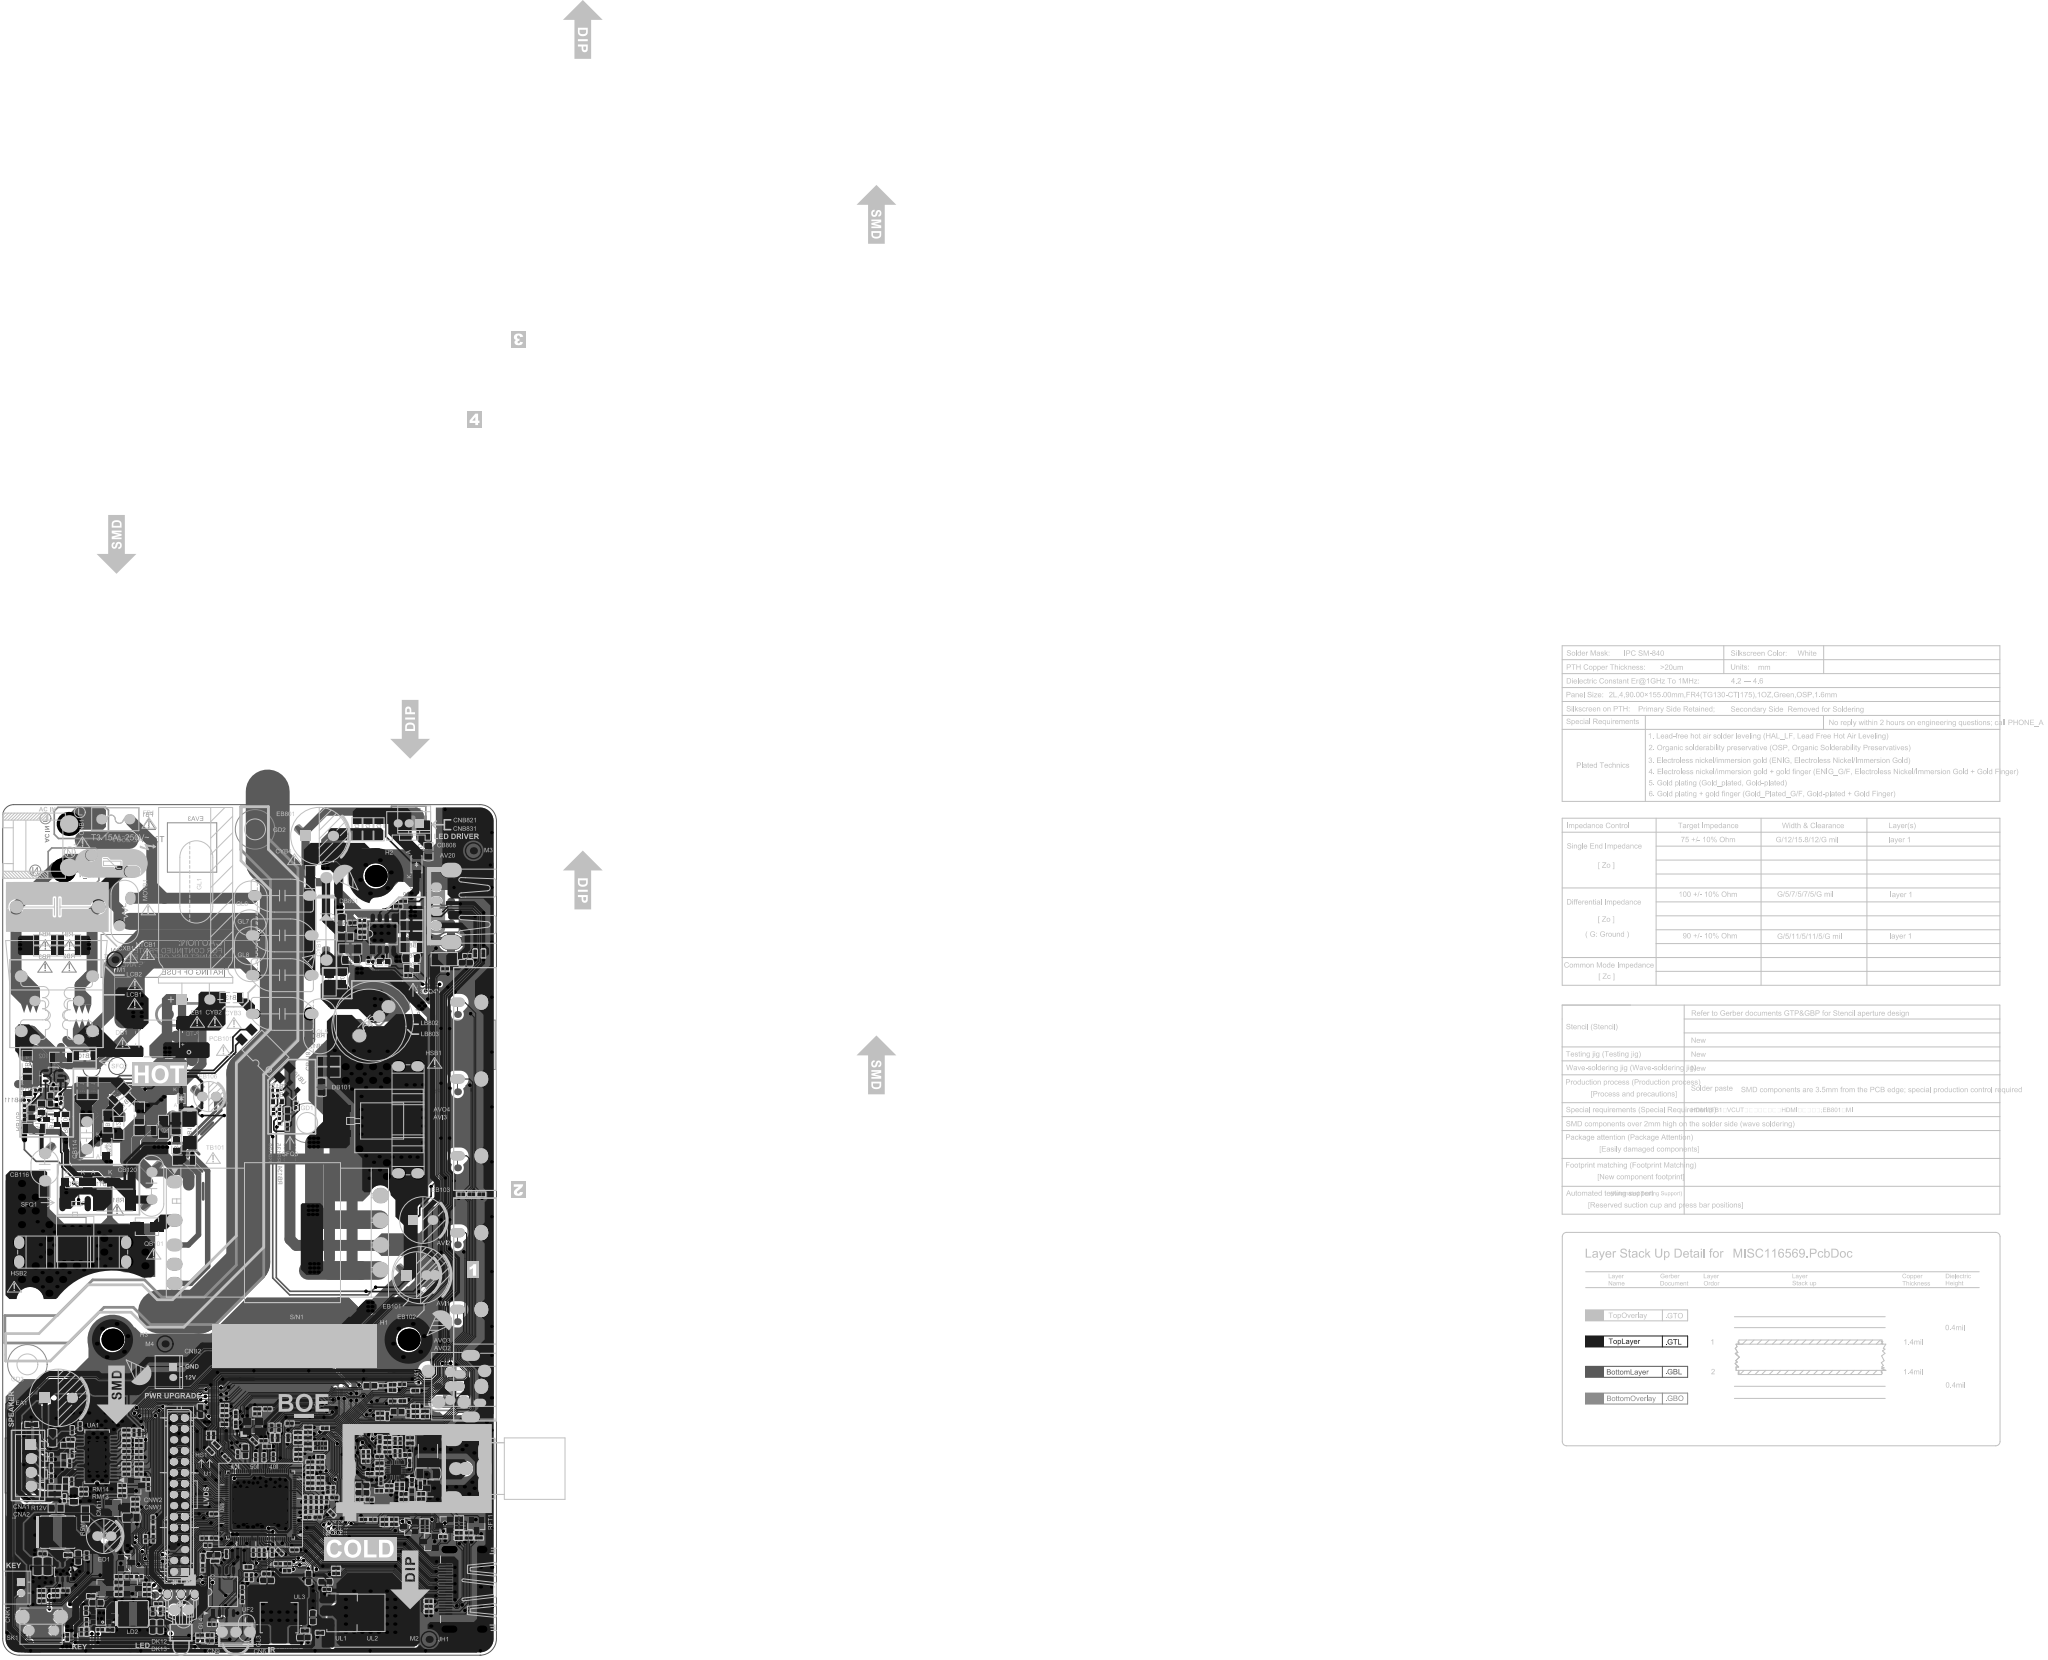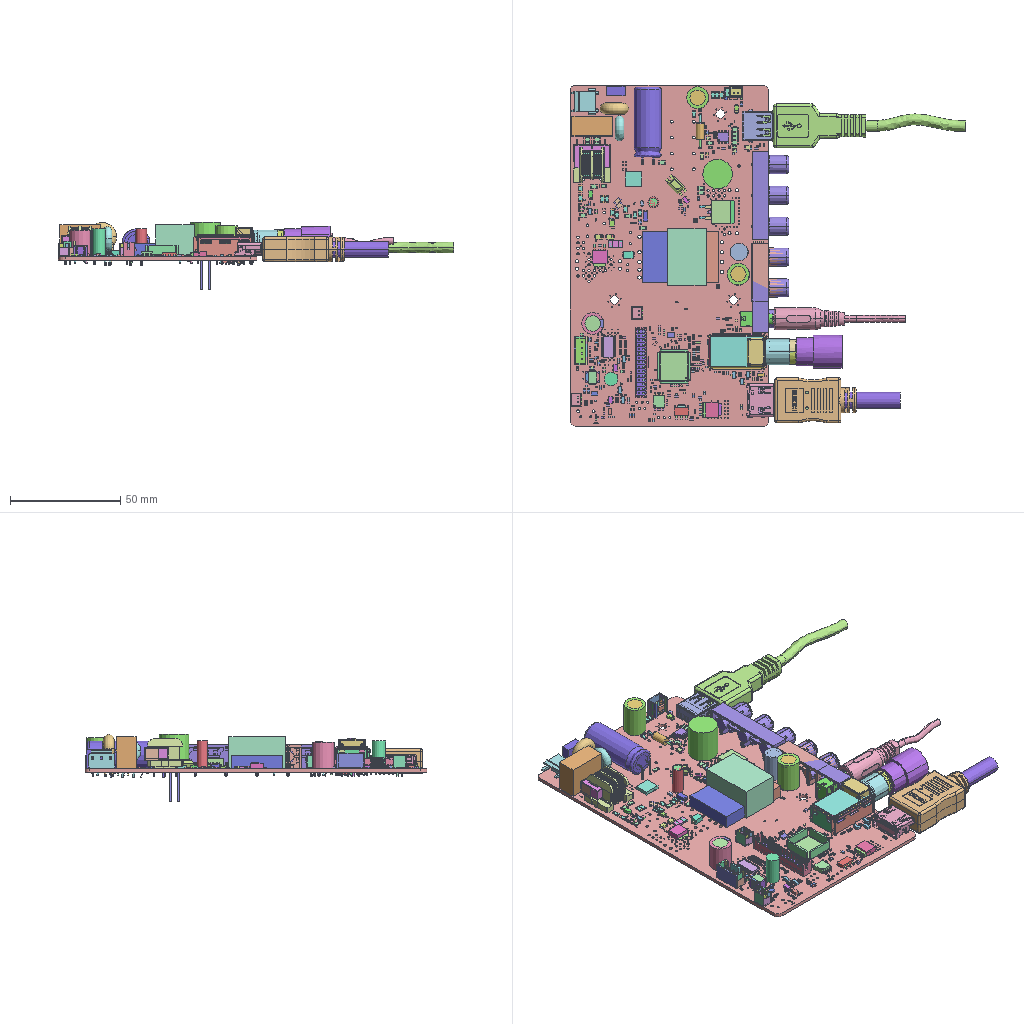Circuit board layout | Altium Designer | box 179.2 x 155 x 30.5 mm
Layer stack:
# Altium Designer layer stack of  (unit mm; dielectric type: 0 none, 1 core, 2 prepreg, 3 surface material)
index,name,kind,layer,copper_thickness_mm,dielectric_type,dielectric_thickness_mm,dielectric_material,dielectric_constant
0,TopPaste,other,,,,,,
1,TopOverlay,other,,,,,,
2,TopSolder,dielectric,,,3,0.0102,Solder Resist,3.5
3,TopLayer,copper,TopLayer,0.0356,,,,
4,Dielectric1,dielectric,,,1,1.5,FR-4,4.8
5,BottomLayer,copper,BottomLayer,0.0356,,,,
6,BottomSolder,dielectric,,,3,0.0102,Solder Resist,3.5
7,BottomOverlay,other,,,,,,
8,BottomPaste,other,,,,,,
# drill layer pairs: low layer,high layer
drill_pair,TopLayer,BottomLayer
Part placement, first 334 of 528 lines:
Designator,Comment,Layer,Footprint,Center-X(mm),Center-Y(mm),Rotation
DBS8,DOLBY Double-D,BottomLayer,Double-D-SILK,-1655.786,-747.429,180
M4,MARK,TopLayer,MARK,29.604,56.731,0
M1,MARK,TopLayer,MARK,20.475,126.729,0
GL4,Silicone,0.5g,general purpose,60,White,SLD-8854W,XY,TopLayer,Silica_gel-5*3,-1655.786,-747.429,0
GL3,Silicone,0.5g,general purpose,60,White,SLD-8854W,XY,TopLayer,Silica_gel-5*3,-1655.786,-747.429,0
SFQ4,NC/Conformal coating,25kg/Can,Peters,TopLayer,SFQ,-1655.786,-747.429,90
SFQ3,NC/Conformal coating,25kg/Can,Peters,TopLayer,SFQ,-1655.786,-747.429,90
SFQ2,NC/Conformal coating,25kg/Can,Peters,TopLayer,SFQ,-1655.786,-747.429,180
SFQ1,NC/Conformal coating,25kg/Can,Peters,TopLayer,SFQ,-1655.786,-747.429,0
GL6,NC/Silicone,0.5g,general purpose,60,White,SLD-8854W,XY,TopLayer,Silica_gel-10,-1655.786,-747.429,0
GL5,NC/Silicone,0.5g,general purpose,60,White,SLD-8854W,XY,TopLayer,Silica_gel-10,-1655.786,-747.429,180
GL8,NC/Silicone,0.5g,general purpose,60,White,SLD-8854W,XY,TopLayer,Silica_gel-10,-1655.786,-747.429,0
GL7,NC/Silicone,0.5g,general purpose,60,White,SLD-8854W,XY,TopLayer,Silica_gel-10,-1655.786,-747.429,0
CB808,220PF-0805-NPO-±10%-200V,TopLayer,C0805,77.597,146.468,90
CYB4,Y capacitor,CAP Y1,CD,100pF,400VAC,±10%,K,10mm,Y5P,DIP,TP,TDK,TopLayer,CAP13*5-V-10-1,50.964,138.428,360
RB5,NC/Thick-film resistor,RES,1/4W,0ohm,±5%,1206,SMD,TopLayer,R1206SC,56.071,141.798,90
FBA2,NC/0ohm-0603-PCB,TopLayer,R0603SC,5.271,42.024,180
FBA1,NC/0ohm-0603-PCB,TopLayer,R0603SC,9.481,29.401,180
RB109,10Kohm-0402-±1%-1/16W,TopLayer,R0402,13.399,82.283,180
QM12,MOSFET,PMOS,-4.3A,-30V,0.048ohm@ID=-3A@VGS=-4.5V,SOT-23-3L,NCE3407AY,NCEPOWER,TopLayer,SOT-23-1,20.531,26.835,90
TB101,变压器,Transformer,EQ2414,300uH,0.2×1P,26Ts,H14.5MAX,SYEQ2414Z-T012064B(BLACK),DIP,SQ,TopLayer,T/EQ2414*10,50.073,77.006,360
CA26,2200pF-0402-X7R-±10%-50V,TopLayer,C0402,8.877,34.096,90
RK3,1Kohm-0402-±1%-1/16W,TopLayer,R0402,44.42,14.226,270
DU4,NC/Thick-film resistor,TVS diode,DIO ESD,0.1pF,25V,0402,SMD,GESD1005H150CR10GPT,Sunlord,TopLayer,DIODE-S0402,37.841,37.213,315
??U1?,NC/Glue,0.1g,silicone,ZJ,TopLayer,Heat-Shrinkable_Tube,35.865,5.359,90
YPBPR_R/AV_R,DM0,BottomLayer,TP,82.875,74.793,90
YPBPR_L/AV_L,DM0,BottomLayer,TP,82.85,60.785,90
Y_Y_AV_OUT,DM0,BottomLayer,TP,82.901,88.814,90
Y_Pr_ROUT,DM0,BottomLayer,TP,82.901,116.766,90
Y_Pb_LOUT,DM0,BottomLayer,TP,82.901,102.669,90
UL2,NC/LC1117COTR33,TopLayer,TO-252,62.68,7.728,270
UL1,LDO regulator,IC LDO,1A,3.3V,15V,SOT223,SMD,SCJT1117B-3.3V,CJKJ,TopLayer,SOT-223,61.83,7.728,270
UD2,DC-DC converter,IC DCDC,Syn,1.2A,6.0V,1.5MHz,SOT23-5,SMD,TMI3408,TOLL,TopLayer,SOT-23-5,17.899,6.975,90
UD1,DC-DC converter,IC DC-DC,Syn,3A,18V,600KHz,SOT23-6,SMD,TMI3253T,TOLL,TopLayer,TSOT23-6,10.917,15.175,270
UB801,PWM controller,IC PWM Controller,120KHz,SOP-8,SMD,OB33510CPA,ON-Bright,TopLayer,SO-8A,69.362,131.458,90
UB101,PWM controller,IC PWM Controller,100KHZ,SOT23-6,SMD,LD5537B3GL,Leadtrend,TopLayer,SOT-26,9.207,105.6,270
UART_RX,,BottomLayer,TP,72.873,23.254,180
SK1,Tact switch,Tact Switch,160±50gf,7.0×10.3×7.0mm,DIP,106520070,VAST,TopLayer,KEY-HD-6,6.996,5.75,0
RU4,Thick-film resistor,RES,1/16W,0ohm,±1%,0402,SMD,TopLayer,R0402,80.64,125.07,180
RT15,Thick-film resistor,RES,1/16W,100ohm,±1%,0402,SMD,TopLayer,R0402,72.436,39.048,90
RT14,Thick-film resistor,RES,1/16W,100ohm,±1%,0402,SMD,TopLayer,R0402,71.521,39.048,90
RT10,Thick-film resistor,RES,1/16W,100ohm,±1%,0402,SMD,TopLayer,R0402,65.724,36.676,90
RPV7,Resistor array,RES ARRAY,1/16W,4×4.7Kohm,±5%,0402,SMD,TopLayer,RA0402,76.901,23.608,360
RPV5,Resistor array,RES ARRAY,1/16W,4×10Kohm,±5%,0402,SMD,TopLayer,RA0402,57.937,38.199,90
RO18,NC/Thick-film resistor,RES,1/16W,75ohm,±1%,0402,SMD,TopLayer,R0402,56.071,34.194,180
RO17,NC/0ohm-0402-±5%-1/16W,TopLayer,R0402,57.868,35.204,360
RM4,Thick-film resistor,RES,1/16W,100Kohm,±1%,0402,SMD,TopLayer,R0402,23.055,14.313,180
RM3,4K7ohm-0402-±1%-1/16W,TopLayer,R0402,24.842,14.313,180
RM2,4K7ohm-0402-±1%-1/16W,TopLayer,R0402,21.135,14.313,180
RK19,1Kohm-0402-±1%-1/16W,TopLayer,R0402,36.482,15.941,90
RK18,22ohm-0402-±1%-1/16W,TopLayer,R0402,35.981,2.657,180
RI18,75ohm-0402-±1%-1/16W,TopLayer,R0402,57.921,32.334,180
RH89,100ohm-0402-±1%-1/16W,TopLayer,R0402,51.906,16.652,180
RH88,100ohm-0402-±1%-1/16W,TopLayer,R0402,71.305,24.778,360
RH59,1Kohm-0402-±1%-1/16W,TopLayer,R0402,80.234,21.605,180
RFT4,NC/RF shield can,RF SHLED,Single,H,F,T14.5,CH6.3,whole,25.0×14.5×10.0mm,DIP,T-14.5×25×10-F14.5-LHD,TopLayer,T-14.5¡Á25¡Á10-F14.5,75.5,34,90
RFT3,NC/T-25×14.5×9-IEC14.5-LHD (3 pins),TopLayer,T-25¡Á14.5¡Á9-IEC14.5-LHD-1,75.5,34,90
RFT2,NC/RF shield can,RF SHLED,Single,H,IEC,T14.5,CH6.3,whole,14.5×25×9,DIP,122010461,VAST,TopLayer,T-14.5¡Á25¡Á9.0-IEC14.5,75.5,34,90
RFT1,RF jack,RF JACK,H,IEC,T14.5,CH6.3,12.4×13.2×7.7mm,DIP,LHD-020 assembly,LHD,TopLayer,ANT-IEC14.5-H-4,84.825,34,90
RF25,Thick-film resistor,RES,1/16W,1.3Kohm,±1%,0402,SMD,TopLayer,R0402,46.376,43.97,180
RD9,Thick-film resistor,RES,1/16W,12Kohm,±1%,0402,SMD,TopLayer,R0402,14.308,4.27,90
RD8,Thick-film resistor,RES,1/16W,13Kohm,±1%,0402,SMD,TopLayer,R0402,15.261,6.083,90
RD7,Thick-film resistor,RES,1/16W,100Kohm,±1%,0402,SMD,TopLayer,R0402,17.782,4.638,180
RD6,NC/?,TopLayer,R0402,9.629,11.773,360
RD5,Thick-film resistor,RES,1/16W,10.5Kohm,±1%,0402,SMD,TopLayer,R0402,7.076,11.773,360
RD3,Thick-film resistor,RES,1/16W,60.4Kohm,±1%,0402,SMD,TopLayer,R0402,7.076,10.858,180
RD1,100Kohm-0402-±1%-1/16W,TopLayer,R0402,9.629,10.858,360
RB839,2R2ohm-1206-±1%-1/4W,TopLayer,R1206,68.591,150.512,270
RB838,2R2ohm-1206-±1%-1/4W,TopLayer,R1206,66.589,150.512,90
RB837,1R6ohm-1206-±1%-1/4W,TopLayer,R1206,64.586,150.512,90
RB820,0R1ohm-1206-±1%-1/4W,TopLayer,R1206,74.493,130.963,180
RB819,0R1ohm-1206-±1%-1/4W,TopLayer,R1206,74.493,132.946,180
RB818,0R2ohm-1206-±1%-1/4W,TopLayer,R1206,74.493,134.928,180
RB816,Thick-film resistor,RES,1/8W,10ohm,±1%,0805,SMD,TopLayer,R0805,74.557,125.146,180
RB814,Thick-film resistor,RES,1/8W,390Kohm,±1%,0805-Auto,SMD,TopLayer,R0805,62.505,130.899,180
RB812,Thick-film resistor,RES,1/4W,10ohm,±1%,1206,SMD,TopLayer,R1206,63.354,128.702,180
RB810,Thick-film resistor,RES,1/4W,10ohm,±1%,1206,SMD,TopLayer,R1206,74.493,128.981,360
RB805,Thick-film resistor,RES,1/16W,100ohm,±1%,0402,SMD,TopLayer,R0402,72.987,137.427,360
RB804,NC/10Kohm-0402-±5%-1/16W,TopLayer,R0402,65.54,133.922,180
RB803,10Kohm-0402-±1%-1/16W,TopLayer,R0402,65.54,130.835,360
RB801,Thick-film resistor,RES,1/16W,100ohm,±1%,0402,SMD,TopLayer,R0402,73.915,123.888,180
RB148,Thick-film resistor,RES,2W,0.36ohm,±5%,2512,SMD,TopLayer,R2512-1,20.434,82.944,180
RB135,18Kohm-0402-±1%-1/16W,TopLayer,R0402,50.516,99.092,270
RB134,4K7ohm-0402-±1%-1/16W,TopLayer,R0402,50.503,97.365,90
RB130,Thick-film resistor,RES,1/4W,20ohm,±1%,1206,SMD,TopLayer,R1206,41.689,119.842,360
RB128,Thick-film resistor,RES,1/4W,100Kohm,±1%,1206-Auto,SMD,TopLayer,R1206,22.123,100.457,45
RB127,Thick-film resistor,RES,1/4W,100Kohm,±1%,1206-Auto,SMD,TopLayer,R1206,21.161,96.094,90
RB126,Thick-film resistor,RES,1/4W,100Kohm,±1%,1206-Auto,SMD,TopLayer,R1206,21.285,102.413,45
RB125,Thick-film resistor,RES,1/4W,100Kohm,±1%,1206-Auto,SMD,TopLayer,R1206,19.168,97.262,90
RB124,47ohm-1206-±5%-1/4W,TopLayer,R1206,59.413,108.246,360
RB123,47ohm-1206-±5%-1/4W,TopLayer,R1206,59.413,106.265,360
RB118,Thick-film resistor,RES,1/4W,10ohm,±1%,1206,SMD,TopLayer,R1206,14.488,103.347,90
RB117,Thick-film resistor,RES,1/4W,10ohm,±1%,1206,SMD,TopLayer,R1206,16.472,103.347,90
RB116,NC/10ohm-1206-±5%-1/4W,TopLayer,R1206,31.598,96.926,270
RB114,4R7ohm-1206-±1%-1/4W,TopLayer,R1206,33.059,90.208,360
RB107,20ohm-0805-±5%-1/8W,TopLayer,R0805,7.087,99.682,270
RB106,68ohm-0805-±5%-1/8W,TopLayer,R0805,11.455,97.638,270
RB105,510ohm-0402-±1%-1/16W,TopLayer,R0402,3.975,97.987,270
RB103,6K8ohm-0402-±1%-1/16W,TopLayer,R0402,3.975,99.695,270
RB102,Thick-film resistor,RES,1/4W,330Kohm,±1%,1206,SMD,TopLayer,R1206,10.631,108.95,180
RB101,Thick-film resistor,RES,1/4W,330Kohm,±1%,1206,SMD,TopLayer,R1206,14.96,109.24,180
RB4,1M2ohm-1206-±5%-1/4W,TopLayer,R1206,7.73,130.345,180
RB3,1M2ohm-1206-±5%-1/4W,TopLayer,R1206,7.73,128.351,180
RB2,1M2ohm-1206-±5%-1/4W,TopLayer,R1206,12.103,128.347,180
RB1,1M2ohm-1206-±5%-1/4W,TopLayer,R1206,12.103,130.341,180
RA34,NC/Thick-film resistor,RES,1/16W,180ohm,±1%,0402,SMD,TopLayer,R0402,73.901,44.025,90
RA33,NC/Thick-film resistor,RES,1/16W,180ohm,±1%,0402,SMD,TopLayer,R0402,69.319,49.088,360
RA32,NC/1Kohm-0402-±1%-1/16W,TopLayer,R0402,72.79,49.378,180
RA31,NC/1Kohm-0402-±1%-1/16W,TopLayer,R0402,75.217,44.44,180
QM2,MOSFET,PMOS,-4.4A,-30V,0.046ohm@ID=-4A@VGS=-4.5V,SOT-23,NCE3401AY,NCEPOWER,TopLayer,SOT-23-1,18.245,12.205,270
QM1,General-purpose transistor,Dynatron,NPN,0.2A,40V,30-300,SOT-23,LMBT3904LT1G,LRC,TopLayer,SOT-23,22.513,16.828,90
QH5,General-purpose transistor,Dynatron,NPN,0.2A,40V,30-300,SOT-23,LMBT3904LT1G,LRC,TopLayer,SOT-23,77.744,20.627,270
QH4,General-purpose transistor,Dynatron,NPN,0.2A,40V,30-300,SOT-23,LMBT3904LT1G,LRC,TopLayer,SOT-23,74.091,23.419,270
QH3,General-purpose transistor,Dynatron,NPN,0.2A,40V,30-300,SOT-23,LMBT3904LT1G,LRC,TopLayer,SOT-23,80.564,23.688,270
QB101,MOSFET,NMOS,5A,650V,0.8ohm@ID=2.5A@VGS=10V,TO-252,SVS5N70D,SL,TopLayer,TO-252-GDS,13.207,78.683,180
PWM_REF,NC/TEST,BottomLayer,TP_BL,78.156,122.784,270
NTCB1,NTC thermistor,RES NTC,2.4W,5A,2.5ohm,±20%,S,5.0mm,10mm,DIP,FH,TopLayer,NTC(10*5)-V5,22.244,135.447,90
MOVB1,NC/Varistor,VARISTOR,128J,680V,4000A,S,7.5mm,10mm,DIP,Thinking,TopLayer,VR(13*5)-V-7.5,19.909,144.297,360
ML1,NC/Latest Mylar sheet,TopLayer,Mylar,-1655.786,-747.429,90
LED_R,TEST  SL,BottomLayer,TP,28.951,8.245,180
LED_G,TEST  SL,BottomLayer,TP,27.764,11.001,180
LD3,NC/Power inductor,Power Inductor,4.7uH,±20%,3.3A,DR6.0×4.5,SMD,SWPA6045S4R7MT,Sunlord,TopLayer,L(6.0*4.5)-S,10.007,22.424,180
LD2,Power inductor,Power Inductor,2.2uH,±20%,2A,0.28×1P,DR4.5×3.2,SMD,PIO43-2R2MTP02,FH,TopLayer,L(4.5*3.5)-S,23.757,7.527,180
LD1,Power inductor,Power Inductor,4.7uH,±20%,2.8A,0.32×1P,DR5.8×4.5,SMD,PIO54-4R7MTP02,FH,TopLayer,L(5.8*4.5)-S,10.013,22.424,180
LCB2,NC/SYUU10.5-L002-JM,TopLayer,L/UU10.5/10*13-2,9.793,118.731,90
LCB1,共模电感,Common Choke,UU9.8,20mH MIN,0.27×1P,86Ts,H14.0MAX,SYUU9.8-L002,DIP,CK,TopLayer,L/LC4/UU9.8/7*8-H,9.793,115.731,180
LB803,NC/Differential-mode inductor,Inductor,DR12×14,68uH,0.45,20Ts,H13.5MAX,SYDR1214-L068uA,DIP,Soldier,TopLayer,L(13.5*15.5)-V-5,66.761,114.633,45
LB802,Differential-mode inductor,Inductor,DR12×12,70uH,0.15×12P,38.5Ts,H13.5MAX,SYDR1212-L070uA,DIP,EDL,TopLayer,L/LC2/15*14.5-V7.5,67.592,115.545,45
L6,NC/0ohm-0402-PCB,TopLayer,R0402SC,66.899,33.086,0
K0,TEST  SL,BottomLayer,TP,4.77,2.25,180
JH1,HDMI jack,HDMI Jack,H,SMD,161031041(hull-SPCC ),VAST,TopLayer,HDMI-HS-1,84.28,12.001,90
IR_IN,TEST  SL,BottomLayer,TP,39.962,6.403,180
High Voltage,High Voltage,TopLayer,High_Voltage,-1655.786,-747.429,90
H3,Location hole,TopLayer,ASSE4.0C-3,19.95,57.352,0
H2,Location hole,TopLayer,ASSE4.0C-3,67.95,141.854,0
H1,Location hole,TopLayer,ASSE4.0C-3,73.95,57.352,0
GL1,Silicone,0.5g,general purpose,60,White,SLD-8854W,XY,TopLayer,Silica_gel-15,-1655.786,-747.429,180
GD3,7.00×8.35mm-Nylon-White-WQM,TopLayer,Fixed,4.5,53,0
GD2,7.00×8.35mm-Nylon-White-WQM,TopLayer,Fixed,46,150.5,0
GD1,7.00×8.35mm-Nylon-White-WQM,TopLayer,Fixed,55.5,97,0
FU1,NC/NSMD110(1206-1.1A),TopLayer,FUSE1.1A-S,80.488,126.848,180
FT2,Ferrite bead,BEAD,1000ohm,0402,300mA,SMD,TRAY,CBM100505U102T,FH,TopLayer,L0402,68.62,29.962,180
EVA3,NC/7×7×3mm-C-4305 fire-retardant foam-Black,BottomLayer,EVA(7*7*3),-1655.786,-747.429,180
EVA2,NC/7×7×3mm-C-4305 fire-retardant foam-Black,BottomLayer,EVA(7*7*3),-1655.786,-747.429,180
EVA1,NC/7×7×3mm-C-4305 fire-retardant foam-Black,BottomLayer,EVA(7*7*3),-1655.786,-747.429,180
ED1,Aluminum electrolytic capacitor,CAP AL,10V,470uF,±20%,PKZH,P,2.5mm,6.3×11,DIP,TP,Koshin,TopLayer,EC(6.3*11)-V-2.5,18.443,21.262,360
EB801,Aluminum electrolytic capacitor,CAP AL,100V,47uF,±20%,LD,PKLW,P,5.0mm,10×12.5,DIP,TP,Koshin,TopLayer,EC(10*12.5)-V-5,57.704,149.299,360
EB106,Aluminum electrolytic capacitor,CAP AL,50V,10uF,±20%,LF,PKZF,P,2.5mm,5×11,DIP,TP,Koshin,TopLayer,EC(5*11)-V-2.5,37.561,101.41,360
EB101,Aluminum electrolytic capacitor,CAP AL,16V,270uF,±20%,SP,RP,S,3.5mm,8×11,DIP,Elite,TopLayer,EC(8*11)-V-3.5,75.437,69.266,360
EB1,Aluminum electrolytic capacitor,CAP AL,400V,47uF,±20%,KY,BW,5.0mm,13×30,DIP,CapXon,TopLayer,EC(13*30)-H-5,35.166,119.484,180
EA1,Aluminum electrolytic capacitor,CAP AL,16V,470uF,±20%,PKRM,P,5.0mm,10×12.5,DIP,TP,Koshin,TopLayer,EC(10*12)-V-5,10.123,46.889,360
DV5,NC/AVLC18S02003,TopLayer,DIODE-S0402,87.257,83.987,180
DV4,NC/AVLC18S02003,TopLayer,DIODE-S0402,83.555,83.987,360
DV3,NC/AVLC18S02003,TopLayer,DIODE-S0402,85.453,83.987,180
DU2,NC/Thick-film resistor,TVS diode,DIO ESD,0.1pF,25V,0402,SMD,GESD1005H150CR10GPT,Sunlord,TopLayer,DIODE-S0402,86.126,127.876,90
DU1,NC/Thick-film resistor,TVS diode,DIO ESD,0.1pF,25V,0402,SMD,GESD1005H150CR10GPT,Sunlord,TopLayer,DIODE-S0402,87.625,127.876,90
DP0,DM0,BottomLayer,TP,81.656,137.417,180
DM0,DM0,BottomLayer,TP,81.656,135.417,180
DK13,Light-emitting diode,Double LED,R/G,30mA,700/450mcd,625/570nm,2.1/2.1V,F3×5.3mm,DIP,WEJ3290C-R3H8-BC,WEJ,TopLayer,LED-HD-5,32.503,11.129,0
DK12,NC/Light-emitting diode,Single LED,RED,25mA,28mcd,638nm,1.9V,f3.85×5.4mm,DIP,HL,TopLayer,LED-HD-6,32.505,8.274,0
DI11,NC/AVLC18S02003,TopLayer,DIODE-S0402,42.489,43.855,90
DI10,NC/AVLC18S02003,TopLayer,DIODE-S0402,42.489,42.052,90
DI3,NC/AIES12U020R2,TopLayer,DIODE-S0402,75.217,48.224,180
DI2,NC/AIES12U020R2,TopLayer,DIODE-S0402,76.988,43.513,180
DI1,NC/AIES12U020R2,TopLayer,DIODE-S0402,71.033,48.313,360
DB804,Rectifier diode,DIO FRD S,1.2A,800V,SOD-123FL,SMD,F1K,YJ,TopLayer,DIODE-S-14,75.433,144.12,90
DB801,Schottky diode,DIO SBD S,2A,100V,DO-15,DIP,SR2100,YJ,TopLayer,D2-H-15,58.929,134.186,90
DB111,Switching diode,DIO SW D1,215mA,85V,SOT-23,SMD,KAV70,KEXIN,TopLayer,SO-23,8.991,97.612,270
DB110,Rectifier diode,DIO FRD S,1.2A,800V,SOD-123FL,SMD,F1K,YJ,TopLayer,DIODE-S-14,18.021,86.198,180
DB109,Rectifier diode,DIO FRD S,1.2A,800V,SOD-123FL,SMD,F1K,YJ,TopLayer,DIODE-S-14,13.006,86.198,180
DB106,Rectifier diode,DIO FRD S,1.2A,800V,eSGA,SMD,R12K,GOOD-ARK,TopLayer,DIODE-S-14,18.898,92.635,270
DB104,Rectifier diode,DIO SI S,1A,1000V,SMAF,SMD,M7F,YJ,TopLayer,DIODE-S-1,34.05,95.658,90
DB101,Schottky diode,DIO SBD D1,10A,150V,TO-263,SMD,HBR10150SS,JLHW,TopLayer,D2PAK3,65.459,97.357,180
DB1,Bridge rectifier,DIO BRD,3A,800V,YBS,SMD,YBS3010A,YJ,TopLayer,B/YBS3010A,28.545,112.395,270
DA33,NC/NC?,TopLayer,DIODE-S0402,72.88,46.319,180
DA32,NC/NC?,TopLayer,DIODE-S0402,71.033,49.291,360
DA31,NC/NC?,TopLayer,DIODE-S0402,75.217,45.38,180
D102,NC/NC?,TopLayer,DIODE-S0402,44.755,16.081,360
D101,NC/NC?,TopLayer,DIODE-S0402,51.798,15.42,360
CYB3,Y capacitor,CAP Y1,CD,470pF,400VAC,±10%,KS,10mm,Y5P,DIP,Wansheng,TopLayer,CAP13*5-V-10-1,50.964,116.874,360
CYB2,Y capacitor,CAP Y1,CD,470pF,400VAC,±10%,KS,10mm,Y5P,DIP,Wansheng,TopLayer,CAP13*5-V-10-1,50.964,123.924,360
CYB1,Y capacitor,CAP Y1,CD,470pF,400VAC,±10%,KS,10mm,Y5P,DIP,Wansheng,TopLayer,CAP13*5-V-10-1,50.964,131.176,360
CXB1,X capacitor,CAP X2,MP,280VAC,0.47uF,±10%,S,15mm-Mini,PC,DIP,JH,TopLayer,CAP18*8.5-V-15,9.931,136.373,180
CVBS_IN,DM0,BottomLayer,TP,79.269,49.024,180
CU2,NC/10uF-0603-X5R-±20%-6.3V,TopLayer,C0603,84.43,126.187,360
CU1,1uF-0402-X5R-±20%-6.3V,TopLayer,C0402,84.698,127.419,360
CT52,NC/10uF-0603-X5R-±20%-6.3V,TopLayer,C0603,65.583,30.952,360
CT36,1uF-0402-X5R-±20%-6.3V,TopLayer,C0402,74.248,38.608,180
CT34,Ceramic capacitor,CAP MC,50V,18pF,±5%,NPO,0402,SMD,TP,TopLayer,C0402,49.002,41.456,270
CT33,Ceramic capacitor,CAP MC,50V,18pF,±5%,NPO,0402,SMD,TP,TopLayer,C0402,50.31,41.456,90
CT23,NC/0.1uF-0402-X5R-±20%-16V,TopLayer,C0402,73.781,36.487,360
CT16,Ceramic capacitor,CAP MC,16V,0.1uF,±10%,X7R,0402,SMD,TP,TopLayer,C0402,50.127,39.605,90
CT6,Ceramic capacitor,CAP MC,50V,2pF,±0.25pF,NPO,0402,SMD,TP,TopLayer,C0402,73.065,29.365,360
CT5,NC/Ceramic capacitor,CAP MC,50V,120pF,±5%,NPO,0402,SMD,TP,TopLayer,C0402,74.595,31.537,90
CT4,Thick-film resistor,RES,1/16W,0ohm,±1%,0402,SMD,TopLayer,C0402,76.271,28.45,360
CT3,Ceramic capacitor,CAP MC,1KV,220pF,±5%,NPO,1206,SMD,TP,TopLayer,C1206,77.503,33.111,360
CT2,NC/0.1uF-0402-X5R-±20%-16V,TopLayer,C0402,66.895,28.361,180
CO18,NC/100pF-0402-X7R-±10%-50V,TopLayer,C0402,57.868,34.194,180
CNB831,Connector socket,connect jack,3Pin,D2.0,D,SNAP,L=2.8mm,DIP,CNJST,TopLayer,SIP3/2.0D-3,74.002,151.591,180
CNB821,Connector socket,connect jack,2Pin,D2.0,D,L=3.4mm,DIP,BOOM,TopLayer,SIP2/2.0D-1,75.002,151.591,180
CNB2,Connector socket,connect jack,2Pin,D2.0,D,L=3.4mm,DIP,BOOM,TopLayer,SIP2/2.0D-1,30.988,51.609,270
CNB1,连接插座,connect jack,2Pin,D7.92,L,SNAP,Fool-proofing,nature,L=2.8mm(11mm),DIP,A3962AW-3P2-A5WA-P-D(针长11.0mm),CNJST,TopLayer,CON2-H7.92,12.023,147.524,360
CM8,NC/0.1uF-0402-X7R-±20%-16V,TopLayer,C0402,24.15,26.53,180
CM7,NC/10uF-0805-X5R-±20%-16V,TopLayer,C0805,23.489,25.07,360
CM3,NC/0.022uF-0402-X7R-±10%-16V,TopLayer,C0402,21.134,12.141,180
CM2,NC/0.1uF-0402-X5R-±20%-16V,TopLayer,C0402,16.111,10.782,180
CM1,Ceramic capacitor,CAP MC,16V,0.1uF,±10%,X7R,0402,SMD,TP,TopLayer,C0402,21.134,13.266,180
CL14,1uF-0402-X5R-±20%-6.3V,TopLayer,C0402,48.056,14.861,360
CL13,NC/10uF-0603-X5R-±20%-6.3V,TopLayer,C0603,48.179,13.642,360
CL12,Ceramic capacitor,CAP MC,16V,0.1uF,±10%,X7R,0402,SMD,TP,TopLayer,C0402,55.107,4.486,180
CL11,NC/10uF-0603-X5R-±20%-6.3V,TopLayer,C0603,54.935,3.241,180
CL2,Ceramic capacitor,CAP MC,16V,0.1uF,±10%,X7R,0402,SMD,TP,TopLayer,C0402,57.818,4.079,360
CL1,NC/10uF-0603-X5R-±20%-6.3V,TopLayer,C0603,56.54,6.891,270
CK7,NC/Ceramic capacitor,CAP MC,16V,0.1uF,±10%,X7R,0402,SMD,TP,TopLayer,C0402,37.731,2.657,360
CK6,NC/10pF-0402-NPO-±5%-50V,TopLayer,C0402,36.482,17.719,270
CI22,NC/NC/10pF-0402-NPO-±5%-50V,TopLayer,C0402,57.387,25.133,360
CI21,NC/NC/10pF-0402-NPO-±5%-50V,TopLayer,C0402,59.245,30.137,270
CI20,NC/NC/10pF-0402-NPO-±5%-50V,TopLayer,C0402,60.446,28.727,360
CI18,NC/30pF-0402-NPO-±5%-50V,TopLayer,C0402,68.745,39.332,270
CI6,Ceramic capacitor,CAP MC,16V,0.1uF,±10%,X7R,0402,SMD,TP,TopLayer,C0402,55.647,38.572,0
CI5,Ceramic capacitor,CAP MC,16V,0.1uF,±10%,X7R,0402,SMD,TP,TopLayer,C0402,55.647,37.505,0
CI1,0.047uF-0402-X7R-±10%-16V,TopLayer,C0402,56.062,31.355,0
CF30,NC/1000pF-0402-X7R-±10%-50V,TopLayer,C0402,52.294,42.23,360
CF29,NC/1000pF-0402-X7R-±10%-50V,TopLayer,C0402,52.04,39.605,270
CD17,NC/0.1uF-0402-X5R-±20%-16V,TopLayer,C0402,15.197,8.118,90
CD16,10uF-0603-X5R-±20%-6.3V,TopLayer,C0603,17.102,9.563,180
CD15,10uF-0603-X5R-±20%-6.3V,TopLayer,C0603,27.345,5.197,90
CD14,10uF-0603-X5R-±20%-6.3V,TopLayer,C0603,28.729,5.197,90
CD13,NC/0.1uF-0402-X5R-±20%-16V,TopLayer,C0402,27.338,7.991,270
CD12,NC/NC/3300pF-0402-X7R-±10%-50V,TopLayer,C0402,15.299,4.27,270
CD10,NC/10uF-0603-X5R-±20%-6.3V,TopLayer,C0603,38.417,18.275,180
CD9,NC/0.1uF-0402-X5R-±20%-16V,TopLayer,C0402,11.434,11.786,180
CD8,1uF-0402-X5R-±20%-6.3V,TopLayer,C0402,19.575,4.638,180
CD7,10uF-0603-X5R-±20%-6.3V,TopLayer,C0603,13.749,17.788,90
CD6,NC/0.1uF-0402-X5R-±20%-16V,TopLayer,C0402,15.299,18.174,90
CD5,NC/56pF-0402-NPO-±5%-50V,TopLayer,C0402,7.088,9.868,180
CD4,Ceramic capacitor,CAP MC,16V,0.1uF,±10%,X7R,0402,SMD,TP,TopLayer,C0402,11.921,18.25,360
CD3,NC/0.1uF-0402-X5R-±20%-16V,TopLayer,C0402,7.276,18.504,360
CD2,10uF-0805-X5R-±20%-16V,TopLayer,C0805,6.365,16.207,270
CD1,NC/10uF-0805-X5R-±20%-16V,TopLayer,C0805,8.174,16.207,270
CB812,0.033uF-0402-X7R-±10%-16V,TopLayer,C0402,65.54,132.918,180
CB810,220PF-0805-NPO-±10%-200V,TopLayer,C0805,63.469,126.733,360
CB809,220PF-0805-NPO-±10%-200V,TopLayer,C0805,74.481,127.051,180
CB807,100pF-0402-NPO-±5%-50V,TopLayer,C0402,67.076,126.34,360
CB806,1000pF-0402-X7R-±10%-50V,TopLayer,C0402,65.54,131.826,180
CB805,NC/0.1uF-0402-X7R-±10%-16V,TopLayer,C0402,63.745,133.477,180
CB804,4700pF-0402-X7R-±10%-50V,TopLayer,C0402,72.098,136.449,180
CB801,Ceramic capacitor,CAP MC,25V,1uF,±10%,X7R,0603,SMD,TP,TopLayer,C0603,69.456,126.362,180
CB120,NC/Ceramic capacitor,CAP CD,1KV,4700pF,±20%,Y5U,K,5.0mm,DIP,TP,Walsin,TopLayer,CAP10*4.5-V-5,27.114,85.534,90
CB118,1000pF-0805-NPO-±10%-200V,TopLayer,C0805,58.11,103.505,90
CB113,NC/220PF-0805-NPO-±10%-200V,TopLayer,C0805,31.661,92.989,90
CB103,1000pF-0402-X7R-±10%-50V,TopLayer,C0402,10.63,101.041,90
CB102,0.1uF-0603-X7R-±10%-50V,TopLayer,C0603,8.725,101.244,270
CB101,100pF-0402-NPO-±5%-50V,TopLayer,C0402,6.382,103.035,180
CAUTION,CAUTION,BottomLayer,CAUTION,-1655.786,-747.429,180
CA32,NC/10uF-0603-X5R-±20%-6.3V,TopLayer,C0603,72.001,44.375,180
CA31,NC/10uF-0603-X5R-±20%-6.3V,TopLayer,C0603,67,49.075,180
BOE,PCB_NAME2,TopLayer,PCB_NAME,1.529,48.138,90
BB801,Ferrite bead,BEAD,60ohm@100MHz,1206,4A,SMD,TP,PZ3216U600-4R0TF,Sunlord,TopLayer,L1206,59.589,122.682,90
BB101,Ferrite bead,BEAD,50ohm,3.0×4.0,9A,SMD,TP,SMB-302540-K5B-L1,SOLDIER,TopLayer,L(4*3*2.55)-S,26.289,78.092,360
AVO4,NC/RCA jack,RCA Jack,AV3,H,Yellow、White、Red,CH5.5,D14,Seal,DIP,RC075-F03L3BY-A,YUQIU (MI material),TopLayer,AV3-H14-15,85.075,105,90
AVO3,NC/RCA jack,RCA Jack,AV3,H,Orange、White、Red,CH5.5,D14,Seal,DIP,AV3-8.4-15C,JSL,TopLayer,AV3-H14-15,85.075,63,90
AVO2,NC/Optical jack,OPTICAL,H,DIP,DQT-026D-2,DQ,TopLayer,OPTICAL-HD-3,83.4,49.025,90
AVI3,RCA jack,RCA Jack,AV3,H,Green、Blue、Red,CH5.5,D14,Seal,DIP,AV3-8.4-15C,JSL,TopLayer,AV3-H14-15,85.075,105,90
AVI2,NC/RCA jack,RCA Jack,AV2,H,White、Red,CH5.5,D14,Seal,DIP,AV63-02S-0030,QS (MI hand-insert material),TopLayer,AV2-H14-15,85.075,70,90
AVI1,RCA jack,RCA Jack,AV3,H,Yellow、White、Red,CH5.5,D14,Seal,DIP,AV3-8.4-15C,JSL (MI material),TopLayer,AV3-H14-15,85.075,63,90
AV41,NC/Earphone jack,Earphone Jack,H,F3.5,CH7.0,Black,switch,Seal,DIP,PJ-373A,JSL,TopLayer,PHONE-HD-42,82.625,48.9,90
AV20,USB jack,USB Jack,H,Single,flange,DIP,WLUS-050F USB,WLCO,TopLayer,USB1-HD-2,80.395,136.5,90
5V,DM0,BottomLayer,TP,81.656,133.417,180
5V_M,TEST,BottomLayer,TP,36.52,1.93,180
5V_IR,TEST  SL,BottomLayer,TP,45.042,6.391,180
1V8_DDR,TEST,BottomLayer,TP,50.427,3.025,180
DAS1,35.0*5.4mm,TopLayer,DOLBY_AS2,-1655.786,-747.429,180
S/N1,Barcode,TopLayer,BARCODE,53.154,56.375,0
S/N2,Barcode,BottomLayer,BARCODE,52.946,44.901,360
CQC,CQC,TopLayer,CQC,-1655.786,-747.429,360
M2,MARK,TopLayer,MARK,77.737,2.883,0
M3,MARK,TopLayer,MARK,85.801,146.596,0
Manufacture_Info,Manufacture_Info,TopLayer,MANUFACTURE_INFO,19.387,29.134,180
XXXXXXXXXXXXX,PCB_NAME,TopLayer,PCB_NAME,52.984,59.893,90
CO12,NC/1uF-0402-X5R-±20%-6.3V,TopLayer,C0402,55.647,39.652,360
RK13,33Kohm-0402-±1%-1/16W,TopLayer,R0402,26.278,11.979,360
UF2,SPI FLASH chip,IC SPI FLASH,4MB,32Mb,SOIC8,SMD,W25Q32JVSSIQ,Winbond,TopLayer,SOIC8,40.165,11.571,90
RT1,Ferrite bead,BEAD,120ohm,0402,800mA,SMD,TP,CBM100505U121T,FH,TopLayer,R0402,65.07,28.374,360
RF9,4K7ohm-0402-±1%-1/16W,TopLayer,R0402,50.198,16.652,360
RF8,4K7ohm-0402-±1%-1/16W,TopLayer,R0402,71.317,23.863,360
CNA2,NC/4PIN-2.54-D-H-G-with latch-B,TopLayer,SIP4/2.5D-2,5.156,34.575,270
CL4,1uF-0402-X5R-±20%-6.3V,TopLayer,C0402,59.069,11.991,360
CL3,NC/10uF-0603-X5R-±20%-6.3V,TopLayer,C0603,58.822,13.376,360
RF43,4K7ohm-0402-±1%-1/16W,TopLayer,R0402,70.124,38.75,360
RF44,4K7ohm-0402-±1%-1/16W,TopLayer,R0402,70.124,39.652,360
RU5,NC/0ohm-0402-PCB,TopLayer,R0402SC,37.518,40.046,90
RM1,10Kohm-0402-±1%-1/16W,TopLayer,R0402,40.407,42.078,180
CA33,NC/1uF-0402-X5R-±20%-6.3V,TopLayer,C0402,40.41,43.665,180
RA35,NC/47Kohm-0402-±1%-1/16W,TopLayer,R0402,40.419,45.494,180
RA36,NC/10Kohm-0402-±1%-1/16W,TopLayer,R0402,40.413,44.579,360
RI3,33ohm-0402-±1%-1/16W,TopLayer,R0402,57.912,31.369,180
RU3,NC/0ohm-0402-PCB,TopLayer,R0402SC,38.431,40.046,90
RA5,NC/?,TopLayer,GND,53.465,42.23,180
RA4,NC/?,TopLayer,GND,55.425,41.997,180
CF40,Ceramic capacitor,CAP MC,50V,0.01uF,±10%,X7R,0402,SMD,TP,TopLayer,C0402,48.274,44.884,180
RT5,Thick-film resistor,RES,1/16W,51Kohm,±1%,0402,SMD,TopLayer,R0402,74.257,39.611,360
LT4,Ferrite bead,BEAD,1000ohm,0402,300mA,SMD,TRAY,CBM100505U102T,FH,TopLayer,L0402,71.852,30.749,90
LT3,Multilayer inductor,HF Inductor,6.8nH,±5%,0402,SMD,MGCI1005T6N8JT-LF,Sunlord,TopLayer,L0402,72.817,30.749,90
LT2,NC/Multilayer inductor,HF Inductor,270nH,±5%,0603,SMD,HCI1608F-R27J-M,Tai-tech,TopLayer,L0603,74.595,29.238,90
CT21,Ceramic capacitor,CAP MC,16V,0.1uF,±10%,X7R,0402,SMD,TP,TopLayer,C0402,74.181,35.035,90
CT20,Ceramic capacitor,CAP MC,50V,22pF,±5%,NPO,0402,SMD,TP,TopLayer,C0402,72.436,36.794,270
CT19,Ceramic capacitor,CAP MC,50V,22pF,±5%,NPO,0402,SMD,TP,TopLayer,C0402,71.522,36.794,270
CT18,Ceramic capacitor,CAP MC,16V,0.1uF,±10%,X7R,0402,SMD,TP,TopLayer,C0402,70.133,37.046,180
CT17,NC/Ceramic capacitor,CAP MC,50V,1000pF,±10%,X7R,0402,SMD,TP,TopLayer,C0402,70.133,37.848,360
CT15,Ceramic capacitor,CAP MC,16V,0.1uF,±10%,X7R,0402,SMD,TP,TopLayer,C0402,49.136,39.605,270
CT14,NC/Ceramic capacitor,CAP MC,50V,22pF,±5%,NPO,0402,SMD,TP,TopLayer,C0402,68.69,36.21,360
CT10,Ceramic capacitor,CAP MC,16V,0.1uF,±10%,X7R,0402,SMD,TP,TopLayer,C0402,68.943,31.714,270
CT8,Ceramic capacitor,CAP MC,16V,0.1uF,±10%,X7R,0402,SMD,TP,TopLayer,C0402,70.441,30.875,360
DT1,Switching diode,DIO SW D2,200mA,100V,SOT-23,SMD,BAV99,YJ,TopLayer,SO-23,78.201,30.406,270
CF1,Ceramic capacitor,CAP MC,50V,18pF,±5%,NPO,0402,SMD,TP,TopLayer,C0402,45.846,38.965,315
CF4,Ceramic capacitor,CAP MC,50V,18pF,±5%,NPO,0402,SMD,TP,TopLayer,C0402,47.535,39.068,180
CF9,Ceramic capacitor,CAP MC,16V,0.1uF,±10%,X7R,0402,SMD,TP,TopLayer,C0402,40.8,35.918,315
CF10,Ceramic capacitor,CAP MC,16V,0.1uF,±10%,X7R,0402,SMD,TP,TopLayer,C0402,55.207,28.355,90
CF11,Ceramic capacitor,CAP MC,16V,0.1uF,±10%,X7R,0402,SMD,TP,TopLayer,C0402,55.207,26.505,270
CF12,Ceramic capacitor,CAP MC,16V,0.1uF,±10%,X7R,0402,SMD,TP,TopLayer,C0402,49.335,36.197,270
CF13,Ceramic capacitor,CAP MC,16V,0.1uF,±10%,X7R,0402,SMD,TP,TopLayer,C0402,56.071,35.204,180
CF14,Ceramic capacitor,CAP MC,16V,0.1uF,±10%,X7R,0402,SMD,TP,TopLayer,C0402,47.638,36.066,270
CF17,Ceramic capacitor,CAP MC,16V,0.1uF,±10%,X7R,0402,SMD,TP,TopLayer,C0402,46.114,36.066,270
CF19,Ceramic capacitor,CAP MC,16V,0.1uF,±10%,X7R,0402,SMD,TP,TopLayer,C0402,42.85,36.644,90
CF24,1uF-0402-X5R-±20%-6.3V,TopLayer,C0402,50.525,18.792,315
CF26,0.047uF-0402-X7R-±10%-16V,TopLayer,C0402,56.071,32.36,360
CF27,NC/0.1uF-0402-X5R-±20%-16V,TopLayer,C0402,53.867,36.614,180
CF28,1uF-0402-X5R-±20%-6.3V,TopLayer,C0402,53.867,35.7,180
CF31,0.047uF-0402-X7R-±10%-16V,TopLayer,C0402,58.102,28.334,270
CF38,NC/30pF-0402-NPO-±5%-50V,TopLayer,C0402,46.376,44.884,360
CT11,NC/Ceramic capacitor,CAP MC,50V,22pF,±5%,NPO,0402,SMD,TP,Walsin,TopLayer,C0402,68.683,33.079,360
CT12,NC/Ceramic capacitor,CAP MC,50V,27pF,±5%,NPO,0402,SMD,TP,TopLayer,C0402,68.683,33.988,360
Pad and via stacks, first 70 of 278 lines:
# Altium Designer via and pad stacks of  (unit mm). Each distinct definition once, with the count of objects using it.
# via: kind,start_layer,end_layer,hole_mm,diameter_mm,mode(0 simple;1 top-mid-bottom;2 full stack),diameter_per_layer,count,example_net
# pad: kind,layer,hole_mm,hole_type(0 round;1 square;2 slot),plating,top_size,top_shape(1 round;2 rect;3 octagon;9 rounded rect),mid_size,bottom_size,mode,footprint,size_per_layer,count,example
pad,TopOverlay,0,0,plated,1.9x2.55,1,1.9x2.55,1.9x2.55,0,CAP13*5-V-10-1,,8,CYB4.61
pad,TopOverlay,0,0,unplated,2.9x2.9,1,2.9x2.9,2.9x2.9,0,T/EQ2414*10,,4,TB101.0
pad,TopOverlay,0,0,unplated,2.4x3,1,2.4x3,2.4x3,0,T/EQ2414*10,,5,TB101.0
pad,TopOverlay,0,0,plated,1.8x1.8,1,1.8x1.8,1.8x1.8,0,REMOTE-VD-6,,3,CN9.0
pad,TopOverlay,0,0,plated,1.7x1.7,1,1.7x1.7,1.7x1.7,0,REMOTE-VD-9,,3,CN6.0
pad,TopOverlay,0,0,plated,1.905x1.905,1,1.905x1.905,1.905x1.905,0,SIP4/2.54D-1,,3,CNA1.0
pad,TopOverlay,0,0,plated,1.905x1.905,2,1.905x1.905,1.905x1.905,0,SIP4/2.54D-1,,1,CNA1.0
pad,TopOverlay,0,0,plated,1.3x1.3,2,1.3x1.3,1.3x1.3,0,SIP2*15/2.0D-11,,1,CNW2.372
pad,TopOverlay,0,0,plated,1.3x1.3,1,1.3x1.3,1.3x1.3,0,SIP2*15/2.0D-11,,28,CNW2.373
pad,TopOverlay,0,0,plated,1.3x1.3,1,1.3x1.3,1.3x1.3,0,SIP2*15/2.0D-2,,28,CNW1.0
pad,TopOverlay,0,0,plated,1.3x1.3,2,1.3x1.3,1.3x1.3,0,SIP2*15/2.0D-2,,1,CNW1.0
pad,TopOverlay,0,0,plated,1.905x1.905,1,1.905x1.905,1.905x1.905,0,SIP4/2.5D-2,,3,CNA2.0
pad,TopOverlay,0,0,plated,1.905x1.905,2,1.905x1.905,1.905x1.905,0,SIP4/2.5D-2,,1,CNA2.0
pad,TopOverlay,0,0,plated,2.1x1.7,1,2.1x1.7,2.1x1.7,0,USB1-HD-2,,2,AV20.0
pad,TopOverlay,0,0,plated,2.7x3.9,1,2.7x3.9,2.7x3.9,0,USB1-HD-2,,2,AV20.0
pad,TopOverlay,0,0,plated,1.4x2.1,1,1.4x2.1,1.4x2.1,0,USB1-HD-2,,2,AV20.1
pad,TopOverlay,0,0,plated,2.3x2.3,1,2.3x2.3,2.3x2.3,0,PHONE-HD-42,,4,AV41.0
pad,TopOverlay,0,0,plated,2.3x1.5,1,2.3x1.5,2.3x1.5,0,PHONE-HD-42,,2,AV41.0
pad,TopOverlay,0,0,plated,2.7x1.7,1,2.7x1.7,2.7x1.7,0,AV2-H14-15,,2,AVI2.0
pad,TopOverlay,0,0,plated,2.8x2.5,1,2.8x2.5,2.8x2.5,0,AV2-H14-15,,2,AVI2.0
pad,TopOverlay,0,0,plated,2x3.4,1,2x3.4,2x3.4,0,OPTICAL-HD-3,,2,AVO2.0
pad,TopOverlay,0,0,plated,1.778x1.778,1,1.778x1.778,1.778x1.778,0,OPTICAL-HD-3,,3,AVO2.0
pad,TopOverlay,0,0,plated,2.7x1.7,1,2.7x1.7,2.7x1.7,0,AV3-H14-15,,12,AVO4.0
pad,TopOverlay,0,0,plated,2.8x2.5,1,2.8x2.5,2.8x2.5,0,AV3-H14-15,,12,AVO4.0
pad,TopOverlay,0,0,plated,3.2x3.2,1,3.2x3.2,3.2x3.2,0,CON2-H7.92,,2,CNB1.109
pad,TopOverlay,0,0,plated,1.3x1.3,1,1.3x1.3,1.3x1.3,0,SIP2/2.0D-1,,3,CNB821.0
pad,TopOverlay,0,0,plated,1.3x1.3,2,1.3x1.3,1.3x1.3,0,SIP2/2.0D-1,,3,CNB821.0
pad,TopOverlay,0,0,plated,1.5x1.5,2,1.5x1.5,1.5x1.5,0,SIP3/2.0D-3,,1,CNB831.0
pad,TopOverlay,0,0,plated,1.5x1.5,1,1.5x1.5,1.5x1.5,0,SIP3/2.0D-3,,2,CNB831.0
pad,TopOverlay,0,0,plated,2.4x2.4,1,2.4x2.4,2.4x2.4,0,CAP18*8.5-V-15,,2,CXB1.78
pad,TopOverlay,0,0,plated,2.1x2.1,1,2.1x2.1,2.1x2.1,0,D2-H-15,,2,DB801.15
pad,TopOverlay,0,0,plated,1.9x1.9,1,1.9x1.9,1.9x1.9,0,LED-HD-6,,2,DK12.4
pad,TopOverlay,0,0,unplated,1.5x1.7,1,1.5x1.7,1.5x1.7,0,LED-HD-5,,3,DK13.0
pad,TopOverlay,0,0,plated,1.9x1.9,2,1.9x1.9,1.9x1.9,0,EC(10*12)-V-5,,1,EA1.0
pad,TopOverlay,0,0,plated,1.9x1.9,1,1.9x1.9,1.9x1.9,0,EC(10*12)-V-5,,1,EA1.0
pad,TopOverlay,0,0,plated,1.9x1.9,1,1.9x1.9,1.9x1.9,0,EC(13*30)-H-5,,1,EB1.53
pad,TopOverlay,0,0,plated,1.9x1.9,2,1.9x1.9,1.9x1.9,0,EC(13*30)-H-5,,1,EB1.54
pad,TopOverlay,0,0,plated,1.8x1.8,1,1.8x1.8,1.8x1.8,0,EC(8*11)-V-3.5,,2,EB101.1
pad,TopOverlay,0,0,plated,1.8x1.8,2,1.8x1.8,1.8x1.8,0,EC(8*11)-V-3.5,,2,EB101.1
pad,TopOverlay,0,0,unplated,1.8x1.8,1,1.8x1.8,1.8x1.8,0,EC(5*11)-V-2.5,,2,EB106.0
pad,TopOverlay,0,0,plated,1.9x1.9,1,1.9x1.9,1.9x1.9,0,EC(10*12.5)-V-5,,2,EB801.1
pad,TopOverlay,0,0,plated,1.9x1.9,2,1.9x1.9,1.9x1.9,0,EC(10*12.5)-V-5,,2,EB801.1
pad,TopOverlay,0,0,plated,2.4x2.4,1,2.4x2.4,2.4x2.4,0,L/LC2/15*14.5-V7.5,,2,LB802.1
pad,TopOverlay,0,0,plated,2.1x2.1,1,2.1x2.1,2.1x2.1,0,L(13.5*15.5)-V-5,,2,LB803.4
pad,TopOverlay,0,0,plated,1.9x1.9,1,1.9x1.9,1.9x1.9,0,L/LC4/UU9.8/7*8-H,,4,LCB1.17
pad,TopOverlay,0,0,plated,2.2x2.2,1,2.2x2.2,2.2x2.2,0,L/UU10.5/10*13-2,,4,LCB2.4
pad,TopOverlay,0,0,plated,2.1x2.1,1,2.1x2.1,2.1x2.1,0,VR(13*5)-V-7.5,,1,MOVB1.2
pad,TopOverlay,0,0,plated,2.2x3,1,2.2x3,2.2x3,0,VR(13*5)-V-7.5,,1,MOVB1.2
pad,TopOverlay,0,0,plated,2x2,1,2x2,2x2,0,NTC(10*5)-V5,,1,NTCB1.2
pad,TopOverlay,0,0,plated,2.4x1.9,1,2.4x1.9,2.4x1.9,0,NTC(10*5)-V5,,1,NTCB1.3
pad,TopOverlay,0,0,unplated,2.7x4.1,1,2.7x4.1,2.7x4.1,0,ANT-IEC14.5-H-4,,1,RFT1.0
pad,TopOverlay,0,0,unplated,2.5x3.8,1,2.5x3.8,2.5x3.8,0,ANT-IEC14.5-H-4,,2,RFT1.0
pad,TopOverlay,0,0,plated,2.4x2.4,1,2.4x2.4,2.4x2.4,0,ANT-IEC14.5-H-4,,1,RFT1.0
pad,TopOverlay,0,0,plated,2.1x3.8,1,2.1x3.8,2.1x3.8,0,T-14.5\u00A1\u00C125\u00A1\u00C19.0-IEC14.5,,1,RFT2.1
pad,TopOverlay,0,0,plated,2.1x4.1,1,2.1x4.1,2.1x4.1,0,T-14.5\u00A1\u00C125\u00A1\u00C19.0-IEC14.5,,2,RFT2.1
pad,TopOverlay,0,0,plated,1.778x4.1,1,1.778x4.1,1.778x4.1,0,T-14.5\u00A1\u00C125\u00A1\u00C19.0-IEC14.5,,1,RFT2.1
pad,TopOverlay,0,0,plated,2.3x2.3,1,2.3x2.3,2.3x2.3,0,T-14.5\u00A1\u00C125\u00A1\u00C19.0-IEC14.5,,1,RFT2.11
pad,TopOverlay,0,0,plated,2.2x3.8,1,2.2x3.8,2.2x3.8,0,T-25\u00A1\u00C114.5\u00A1\u00C19-IEC14.5-LHD-1,,3,RFT3.5
pad,TopOverlay,0,0,plated,1.778x4.1,1,1.778x4.1,1.778x4.1,0,T-25\u00A1\u00C114.5\u00A1\u00C19-IEC14.5-LHD-1,,1,RFT3.1
pad,TopOverlay,0,0,plated,2.1x4.1,1,2.1x4.1,2.1x4.1,0,T-25\u00A1\u00C114.5\u00A1\u00C19-IEC14.5-LHD-1,,2,RFT3.1
pad,TopOverlay,0,0,plated,2.4x2.4,1,2.4x2.4,2.4x2.4,0,T-25\u00A1\u00C114.5\u00A1\u00C19-IEC14.5-LHD-1,,1,RFT3.0
pad,TopOverlay,0,0,plated,2.1x4.1,1,2.1x4.1,2.1x4.1,0,T-14.5\u00A1\u00C125\u00A1\u00C110-F14.5,,3,RFT4.0
pad,TopOverlay,0,0,plated,1.778x4.1,1,1.778x4.1,1.778x4.1,0,T-14.5\u00A1\u00C125\u00A1\u00C110-F14.5,,1,RFT4.0
pad,TopOverlay,0,0,plated,2.3x2.3,1,2.3x2.3,2.3x2.3,0,T-14.5\u00A1\u00C125\u00A1\u00C110-F14.5,,1,RFT4.0
pad,TopOverlay,0,0,plated,2.5x2.5,1,2.5x2.5,2.5x2.5,0,KEY-HD-6,,2,SK1.0
pad,TopOverlay,0,0,plated,1.8x1.8,1,1.8x1.8,1.8x1.8,0,KEY-HD-6,,2,SK1.0
pad,TopOverlay,0,0,plated,1.9x1.9,1,1.9x1.9,1.9x1.9,0,CAP10*4.5-V-5,,2,CB120.41
Copper pours:
name,layer,net,type(0 solid;1 hatched;2 none)
5,TopLayer,12V,0
12,TopLayer,D_QB101,0
5,TopLayer,DRIM,0
5,TopLayer,NetBB801_2,0
5,TopLayer,GND,0
5,TopLayer,GND,0
5,TopLayer,GND,0
12,TopLayer,GND,0
12,TopLayer,GND,0
12,TopLayer,GND,0
12,TopLayer,GND,0
5,TopLayer,GND,0
12,TopLayer,GND,0
12,TopLayer,L,0
5,TopLayer,N-3,0
12,BottomLayer,SGND,0
12,BottomLayer,GND,0
12,BottomLayer,D_QB101,0
5,BottomLayer,GND,0
12,BottomLayer,GND,0
5,BottomLayer,GND,0
5,BottomLayer,12V,0
Design rules, without the lines most boards share, first 16 of 33 lines:
# Altium Designer design rules of  (exported by Altium Designer, unit mm)
# columns: name | kind | enabled | priority | scope1 | scope2 | descriptor | typed fields (field=value)
NetAntennae | 56 | enabled | 1 | Not (HasFootprint('ANT-7') or HasFootprint('ANT-BLUECORE')) | All | Net Antennae (Tolerance=1.016mm) (Not (HasFootprint('ANT-7') or HasFootprint('ANT-BLUECORE'))) |
Hole2Hole | 52 | disabled | 1 | All | All | Hole To Hole Clearance (Gap=0.457mm) (Disabled)(All),(All) | gap=0.4572
DiffPairsRouting | 51 | enabled | 4 | All | All | Differential Pairs Uncoupled Length using the Gap Constraints (Min=0.254mm) (Max=0.254mm) (Prefered=0.254mm)  and Width Constraints (Min=0.381mm) (Max=0.381mm) (Prefered=0.381mm) (All) |
Height | 50 | enabled | 1 | All | All | Height Constraint (Min=0mm) (Max=25.4mm) (Prefered=12.7mm) (All) | min_height=0 max_height=25.4
TestPointUsage | 44 | enabled | 1 | All | All | Fabrication Testpoint Usage (Valid =One Required, Allow multiple per net=No) (All) |
Testpoint | 43 | enabled | 1 | All | All | Fabrication Testpoint Style (Under Component=Yes) (All) |
HoleSize_VIA | 42 | disabled | 1 | ISVIA | All | Hole Size Constraint (Min=0.2mm) (Max=0.6mm) (Disabled)(ISVIA) |
PermittedLayers | 26 | enabled | 1 | All | All | Permitted Layers - (Top Layer, Bottom Layer) (All) |
SMDToCorner | 23 | disabled | 1 | All | All | SMD To Corner (Distance=0.102mm) (Disabled)(All) |
MinimumAnnularRing | 19 | enabled | 1 | All | All | Minimum Annular Ring (Minimum=0.1mm) (All) |
ViasUnderSMD | 17 | enabled | 1 | All | All | Vias Under SMD Constraint (Allowed=Not Allowed) (All) |
PasteMaskExpansion | 14 | enabled | 1 | All | All | Paste Mask Expansion (Expansion =0mm) (All) | expansion=0
0.25_0.1 | 11 | disabled | 6 | All | All | Routing Via (MinHoleWidth=0.1mm) (MaxHoleWidth=0.1mm) (PreferredHoleWidth=0.1mm) (MinWidth=0.25mm) (MaxWidth=0.25mm) (PreferedWidth=0.25mm) (Disabled)(All) | via_min_hole=0.1 via_max_hole=0.1 via_preferred_diameter=0.25 via_preferred_hole=0.1
0.4_0.2 | 11 | disabled | 5 | All | All | Routing Via (MinHoleWidth=0.2mm) (MaxHoleWidth=0.2mm) (PreferredHoleWidth=0.2mm) (MinWidth=0.4mm) (MaxWidth=0.4mm) (PreferedWidth=0.4mm) (Disabled)(All) | via_min_hole=0.2 via_max_hole=0.2 via_preferred_diameter=0.4 via_preferred_hole=0.2